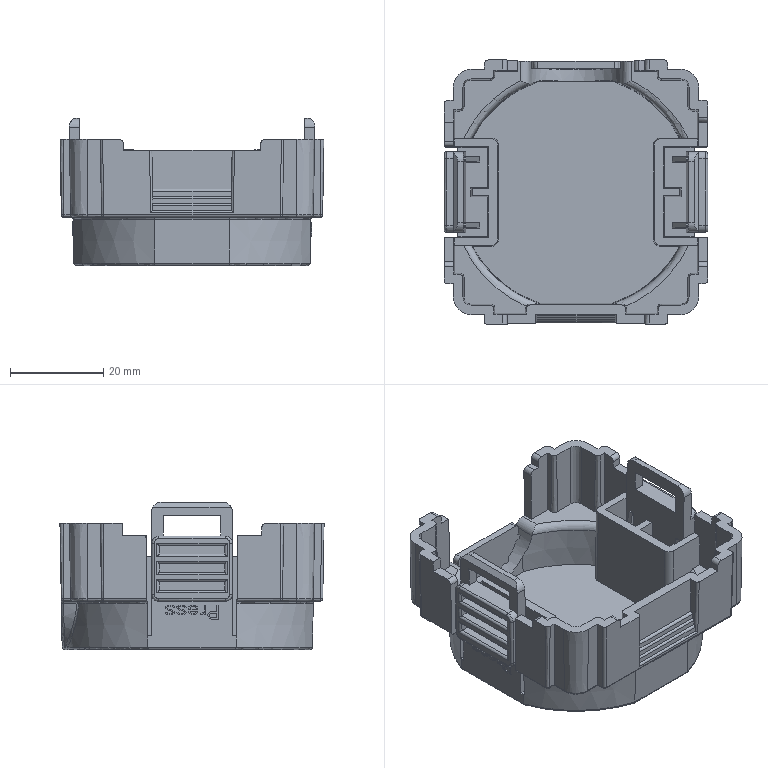Part | NX | features BREP 1 | 1 solid | 2044 faces | box 56.502 x 56.532 x 31.491 mm | volume 17778 mm3 | plane 1848 | cylinder 118 | spline 32 | torus 24 | cone 20 | sphere 2 | commonest cylinder face diameters 1 x67 4 x17 2 x11 18.401 x6 2.8 x4 3 x4